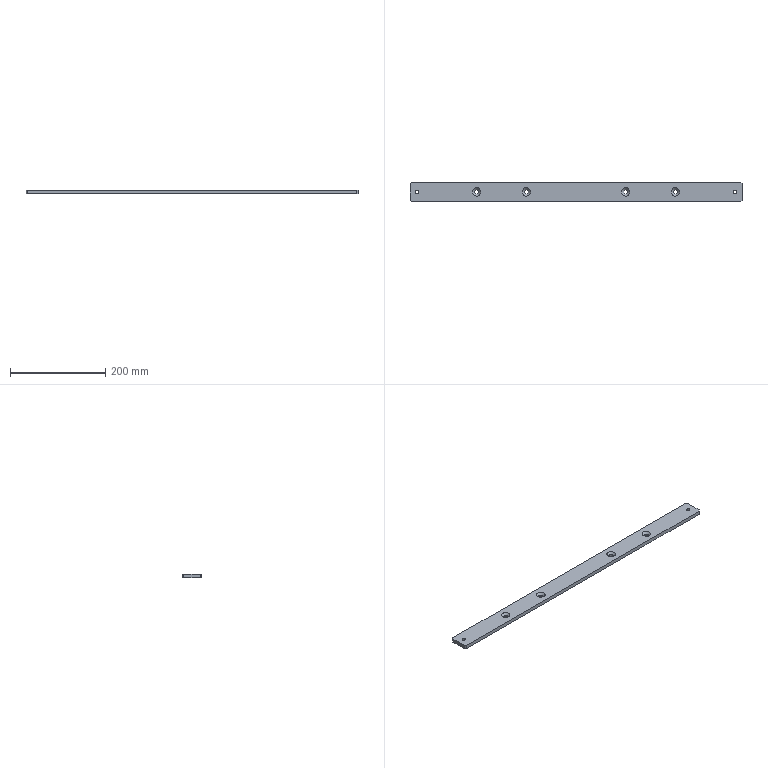Part | STEP file | rectangular profile 40x8-698 | 1 solid | 20 faces | box 698 x 40 x 8 mm | volume 219099 mm3 | spline 10 | plane 10